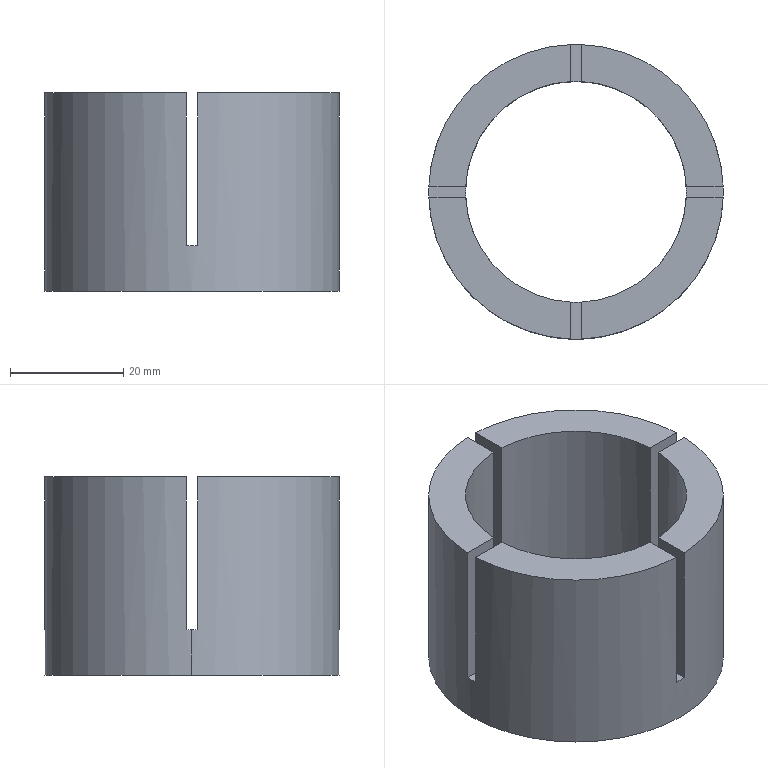Part | SolidWorks | features BaseBody 1, Cut 1 | 1 solid | 21 faces | box 52 x 52 x 35 mm | volume 31115 mm3 | plane 17 | cylinder 4 | commonest cylinder face diameters 39 x2 52 x2
STEP:
#1=CARTESIAN_POINT('',(26.,0.,11.));
#2=VERTEX_POINT('',#1);
#3=CARTESIAN_POINT('',(-26.,0.,11.));
#4=VERTEX_POINT('',#3);
#5=CARTESIAN_POINT('',(0.,0.,11.));
#6=DIRECTION('',(0.,0.,1.));
#7=DIRECTION('',(1.,0.,0.));
#8=AXIS2_PLACEMENT_3D('',#5,#6,#7);
#9=CIRCLE('',#8,26.);
#10=EDGE_CURVE('',#2,#4,#9,.T.);
#11=ORIENTED_EDGE('',*,*,#10,.T.);
#12=CARTESIAN_POINT('',(-26.,0.,19.));
#13=VERTEX_POINT('',#12);
#14=CARTESIAN_POINT('',(-26.,0.,11.));
#15=DIRECTION('',(0.,0.,1.));
#16=VECTOR('',#15,1000.);
#17=LINE('',#14,#16);
#18=EDGE_CURVE('',#4,#13,#17,.T.);
#19=ORIENTED_EDGE('',*,*,#18,.T.);
#20=CARTESIAN_POINT('',(-25.981,1.,19.));
#21=VERTEX_POINT('',#20);
#22=CARTESIAN_POINT('',(0.,0.,19.));
#23=DIRECTION('',(0.,0.,-1.));
#24=DIRECTION('',(1.,0.,0.));
#25=AXIS2_PLACEMENT_3D('',#22,#23,#24);
#26=CIRCLE('',#25,26.);
#27=EDGE_CURVE('',#13,#21,#26,.T.);
#28=ORIENTED_EDGE('',*,*,#27,.T.);
#29=CARTESIAN_POINT('',(-25.981,1.,46.));
#30=VERTEX_POINT('',#29);
#31=CARTESIAN_POINT('',(-25.981,1.,11.));
#32=DIRECTION('',(0.,0.,1.));
#33=VECTOR('',#32,1000.);
#34=LINE('',#31,#33);
#35=EDGE_CURVE('',#21,#30,#34,.T.);
#36=ORIENTED_EDGE('',*,*,#35,.T.);
#37=CARTESIAN_POINT('',(-1.,25.981,46.));
#38=VERTEX_POINT('',#37);
#39=CARTESIAN_POINT('',(0.,0.,46.));
#40=DIRECTION('',(0.,0.,-1.));
#41=DIRECTION('',(1.,0.,0.));
#42=AXIS2_PLACEMENT_3D('',#39,#40,#41);
#43=CIRCLE('',#42,26.);
#44=EDGE_CURVE('',#30,#38,#43,.T.);
#45=ORIENTED_EDGE('',*,*,#44,.T.);
#46=CARTESIAN_POINT('',(-1.,25.981,19.));
#47=VERTEX_POINT('',#46);
#48=CARTESIAN_POINT('',(-1.,25.981,11.));
#49=DIRECTION('',(0.,0.,-1.));
#50=VECTOR('',#49,1000.);
#51=LINE('',#48,#50);
#52=EDGE_CURVE('',#38,#47,#51,.T.);
#53=ORIENTED_EDGE('',*,*,#52,.T.);
#54=CARTESIAN_POINT('',(1.,25.981,19.));
#55=VERTEX_POINT('',#54);
#56=CARTESIAN_POINT('',(0.,0.,19.));
#57=DIRECTION('',(0.,0.,-1.));
#58=DIRECTION('',(1.,0.,0.));
#59=AXIS2_PLACEMENT_3D('',#56,#57,#58);
#60=CIRCLE('',#59,26.);
#61=EDGE_CURVE('',#47,#55,#60,.T.);
#62=ORIENTED_EDGE('',*,*,#61,.T.);
#63=CARTESIAN_POINT('',(1.,25.981,46.));
#64=VERTEX_POINT('',#63);
#65=CARTESIAN_POINT('',(1.,25.981,11.));
#66=DIRECTION('',(0.,0.,1.));
#67=VECTOR('',#66,1000.);
#68=LINE('',#65,#67);
#69=EDGE_CURVE('',#55,#64,#68,.T.);
#70=ORIENTED_EDGE('',*,*,#69,.T.);
#71=CARTESIAN_POINT('',(25.981,1.,46.));
#72=VERTEX_POINT('',#71);
#73=CARTESIAN_POINT('',(0.,0.,46.));
#74=DIRECTION('',(0.,0.,-1.));
#75=DIRECTION('',(1.,0.,0.));
#76=AXIS2_PLACEMENT_3D('',#73,#74,#75);
#77=CIRCLE('',#76,26.);
#78=EDGE_CURVE('',#64,#72,#77,.T.);
#79=ORIENTED_EDGE('',*,*,#78,.T.);
#80=CARTESIAN_POINT('',(25.981,1.,19.));
#81=VERTEX_POINT('',#80);
#82=CARTESIAN_POINT('',(25.981,1.,11.));
#83=DIRECTION('',(0.,0.,-1.));
#84=VECTOR('',#83,1000.);
#85=LINE('',#82,#84);
#86=EDGE_CURVE('',#72,#81,#85,.T.);
#87=ORIENTED_EDGE('',*,*,#86,.T.);
#88=CARTESIAN_POINT('',(26.,0.,19.));
#89=VERTEX_POINT('',#88);
#90=CARTESIAN_POINT('',(0.,0.,19.));
#91=DIRECTION('',(0.,0.,1.));
#92=DIRECTION('',(1.,0.,0.));
#93=AXIS2_PLACEMENT_3D('',#90,#91,#92);
#94=CIRCLE('',#93,26.);
#95=EDGE_CURVE('',#89,#81,#94,.T.);
#96=ORIENTED_EDGE('',*,*,#95,.F.);
#97=CARTESIAN_POINT('',(26.,0.,11.));
#98=DIRECTION('',(0.,0.,1.));
#99=VECTOR('',#98,1000.);
#100=LINE('',#97,#99);
#101=EDGE_CURVE('',#2,#89,#100,.T.);
#102=ORIENTED_EDGE('',*,*,#101,.F.);
#103=EDGE_LOOP('',(#11,#19,#28,#36,#45,#53,#62,#70,#79,#87,#96,#102));
#104=FACE_OUTER_BOUND('',#103,.T.);
#105=CARTESIAN_POINT('',(0.,0.,11.));
#106=DIRECTION('',(0.,0.,1.));
#107=DIRECTION('',(1.,0.,0.));
#108=AXIS2_PLACEMENT_3D('',#105,#106,#107);
#109=CYLINDRICAL_SURFACE('',#108,26.);
#110=ADVANCED_FACE('',(#104),#109,.T.);
#111=CARTESIAN_POINT('',(19.5,0.,11.));
#112=VERTEX_POINT('',#111);
#113=CARTESIAN_POINT('',(-19.5,0.,11.));
#114=VERTEX_POINT('',#113);
#115=CARTESIAN_POINT('',(0.,0.,11.));
#116=DIRECTION('',(0.,0.,-1.));
#117=DIRECTION('',(1.,0.,0.));
#118=AXIS2_PLACEMENT_3D('',#115,#116,#117);
#119=CIRCLE('',#118,19.5);
#120=EDGE_CURVE('',#112,#114,#119,.T.);
#121=ORIENTED_EDGE('',*,*,#120,.T.);
#122=CARTESIAN_POINT('',(-19.5,0.,19.));
#123=VERTEX_POINT('',#122);
#124=CARTESIAN_POINT('',(-19.5,0.,11.));
#125=DIRECTION('',(0.,0.,1.));
#126=VECTOR('',#125,1000.);
#127=LINE('',#124,#126);
#128=EDGE_CURVE('',#114,#123,#127,.T.);
#129=ORIENTED_EDGE('',*,*,#128,.T.);
#130=CARTESIAN_POINT('',(-19.474,-1.,19.));
#131=VERTEX_POINT('',#130);
#132=CARTESIAN_POINT('',(0.,0.,19.));
#133=DIRECTION('',(0.,0.,-1.));
#134=DIRECTION('',(1.,0.,0.));
#135=AXIS2_PLACEMENT_3D('',#132,#133,#134);
#136=CIRCLE('',#135,19.5);
#137=EDGE_CURVE('',#131,#123,#136,.T.);
#138=ORIENTED_EDGE('',*,*,#137,.F.);
#139=CARTESIAN_POINT('',(-19.474,-1.,46.));
#140=VERTEX_POINT('',#139);
#141=CARTESIAN_POINT('',(-19.474,-1.,19.));
#142=DIRECTION('',(0.,0.,-1.));
#143=VECTOR('',#142,1000.);
#144=LINE('',#141,#143);
#145=EDGE_CURVE('',#140,#131,#144,.T.);
#146=ORIENTED_EDGE('',*,*,#145,.F.);
#147=CARTESIAN_POINT('',(-1.,-19.474,46.));
#148=VERTEX_POINT('',#147);
#149=CARTESIAN_POINT('',(0.,0.,46.));
#150=DIRECTION('',(0.,0.,-1.));
#151=DIRECTION('',(1.,0.,0.));
#152=AXIS2_PLACEMENT_3D('',#149,#150,#151);
#153=CIRCLE('',#152,19.5);
#154=EDGE_CURVE('',#148,#140,#153,.T.);
#155=ORIENTED_EDGE('',*,*,#154,.F.);
#156=CARTESIAN_POINT('',(-1.,-19.474,19.));
#157=VERTEX_POINT('',#156);
#158=CARTESIAN_POINT('',(-1.,-19.474,19.));
#159=DIRECTION('',(0.,0.,-1.));
#160=VECTOR('',#159,1000.);
#161=LINE('',#158,#160);
#162=EDGE_CURVE('',#148,#157,#161,.T.);
#163=ORIENTED_EDGE('',*,*,#162,.T.);
#164=CARTESIAN_POINT('',(1.,-19.474,19.));
#165=VERTEX_POINT('',#164);
#166=CARTESIAN_POINT('',(0.,0.,19.));
#167=DIRECTION('',(0.,0.,-1.));
#168=DIRECTION('',(1.,0.,0.));
#169=AXIS2_PLACEMENT_3D('',#166,#167,#168);
#170=CIRCLE('',#169,19.5);
#171=EDGE_CURVE('',#165,#157,#170,.T.);
#172=ORIENTED_EDGE('',*,*,#171,.F.);
#173=CARTESIAN_POINT('',(1.,-19.474,46.));
#174=VERTEX_POINT('',#173);
#175=CARTESIAN_POINT('',(1.,-19.474,19.));
#176=DIRECTION('',(0.,0.,-1.));
#177=VECTOR('',#176,1000.);
#178=LINE('',#175,#177);
#179=EDGE_CURVE('',#174,#165,#178,.T.);
#180=ORIENTED_EDGE('',*,*,#179,.F.);
#181=CARTESIAN_POINT('',(19.474,-1.,46.));
#182=VERTEX_POINT('',#181);
#183=CARTESIAN_POINT('',(0.,0.,46.));
#184=DIRECTION('',(0.,0.,-1.));
#185=DIRECTION('',(1.,0.,0.));
#186=AXIS2_PLACEMENT_3D('',#183,#184,#185);
#187=CIRCLE('',#186,19.5);
#188=EDGE_CURVE('',#182,#174,#187,.T.);
#189=ORIENTED_EDGE('',*,*,#188,.F.);
#190=CARTESIAN_POINT('',(19.474,-1.,19.));
#191=VERTEX_POINT('',#190);
#192=CARTESIAN_POINT('',(19.474,-1.,19.));
#193=DIRECTION('',(0.,0.,1.));
#194=VECTOR('',#193,1000.);
#195=LINE('',#192,#194);
#196=EDGE_CURVE('',#191,#182,#195,.T.);
#197=ORIENTED_EDGE('',*,*,#196,.F.);
#198=CARTESIAN_POINT('',(19.5,0.,19.));
#199=VERTEX_POINT('',#198);
#200=CARTESIAN_POINT('',(0.,0.,19.));
#201=DIRECTION('',(0.,0.,-1.));
#202=DIRECTION('',(1.,0.,0.));
#203=AXIS2_PLACEMENT_3D('',#200,#201,#202);
#204=CIRCLE('',#203,19.5);
#205=EDGE_CURVE('',#199,#191,#204,.T.);
#206=ORIENTED_EDGE('',*,*,#205,.F.);
#207=CARTESIAN_POINT('',(19.5,0.,11.));
#208=DIRECTION('',(0.,0.,1.));
#209=VECTOR('',#208,1000.);
#210=LINE('',#207,#209);
#211=EDGE_CURVE('',#112,#199,#210,.T.);
#212=ORIENTED_EDGE('',*,*,#211,.F.);
#213=EDGE_LOOP('',(#121,#129,#138,#146,#155,#163,#172,#180,#189,#197,#206,#212));
#214=FACE_OUTER_BOUND('',#213,.T.);
#215=CARTESIAN_POINT('',(0.,0.,11.));
#216=DIRECTION('',(0.,0.,1.));
#217=DIRECTION('',(1.,0.,0.));
#218=AXIS2_PLACEMENT_3D('',#215,#216,#217);
#219=CYLINDRICAL_SURFACE('',#218,19.5);
#220=ADVANCED_FACE('',(#214),#219,.F.);
#221=ORIENTED_EDGE('',*,*,#18,.F.);
#222=CARTESIAN_POINT('',(0.,0.,11.));
#223=DIRECTION('',(0.,0.,1.));
#224=DIRECTION('',(1.,0.,0.));
#225=AXIS2_PLACEMENT_3D('',#222,#223,#224);
#226=CIRCLE('',#225,26.);
#227=EDGE_CURVE('',#4,#2,#226,.T.);
#228=ORIENTED_EDGE('',*,*,#227,.T.);
#229=ORIENTED_EDGE('',*,*,#101,.T.);
#230=CARTESIAN_POINT('',(25.981,-1.,19.));
#231=VERTEX_POINT('',#230);
#232=CARTESIAN_POINT('',(0.,0.,19.));
#233=DIRECTION('',(0.,0.,1.));
#234=DIRECTION('',(1.,0.,0.));
#235=AXIS2_PLACEMENT_3D('',#232,#233,#234);
#236=CIRCLE('',#235,26.);
#237=EDGE_CURVE('',#231,#89,#236,.T.);
#238=ORIENTED_EDGE('',*,*,#237,.F.);
#239=CARTESIAN_POINT('',(25.981,-1.,46.));
#240=VERTEX_POINT('',#239);
#241=CARTESIAN_POINT('',(25.981,-1.,11.));
#242=DIRECTION('',(0.,0.,1.));
#243=VECTOR('',#242,1000.);
#244=LINE('',#241,#243);
#245=EDGE_CURVE('',#231,#240,#244,.T.);
#246=ORIENTED_EDGE('',*,*,#245,.T.);
#247=CARTESIAN_POINT('',(1.,-25.981,46.));
#248=VERTEX_POINT('',#247);
#249=CARTESIAN_POINT('',(0.,0.,46.));
#250=DIRECTION('',(0.,0.,-1.));
#251=DIRECTION('',(1.,0.,0.));
#252=AXIS2_PLACEMENT_3D('',#249,#250,#251);
#253=CIRCLE('',#252,26.);
#254=EDGE_CURVE('',#240,#248,#253,.T.);
#255=ORIENTED_EDGE('',*,*,#254,.T.);
#256=CARTESIAN_POINT('',(1.,-25.981,19.));
#257=VERTEX_POINT('',#256);
#258=CARTESIAN_POINT('',(1.,-25.981,11.));
#259=DIRECTION('',(0.,0.,-1.));
#260=VECTOR('',#259,1000.);
#261=LINE('',#258,#260);
#262=EDGE_CURVE('',#248,#257,#261,.T.);
#263=ORIENTED_EDGE('',*,*,#262,.T.);
#264=CARTESIAN_POINT('',(-1.,-25.981,19.));
#265=VERTEX_POINT('',#264);
#266=CARTESIAN_POINT('',(0.,0.,19.));
#267=DIRECTION('',(0.,0.,-1.));
#268=DIRECTION('',(1.,0.,0.));
#269=AXIS2_PLACEMENT_3D('',#266,#267,#268);
#270=CIRCLE('',#269,26.);
#271=EDGE_CURVE('',#257,#265,#270,.T.);
#272=ORIENTED_EDGE('',*,*,#271,.T.);
#273=CARTESIAN_POINT('',(-1.,-25.981,46.));
#274=VERTEX_POINT('',#273);
#275=CARTESIAN_POINT('',(-1.,-25.981,11.));
#276=DIRECTION('',(0.,0.,1.));
#277=VECTOR('',#276,1000.);
#278=LINE('',#275,#277);
#279=EDGE_CURVE('',#265,#274,#278,.T.);
#280=ORIENTED_EDGE('',*,*,#279,.T.);
#281=CARTESIAN_POINT('',(-25.981,-1.,46.));
#282=VERTEX_POINT('',#281);
#283=CARTESIAN_POINT('',(0.,0.,46.));
#284=DIRECTION('',(0.,0.,-1.));
#285=DIRECTION('',(1.,0.,0.));
#286=AXIS2_PLACEMENT_3D('',#283,#284,#285);
#287=CIRCLE('',#286,26.);
#288=EDGE_CURVE('',#274,#282,#287,.T.);
#289=ORIENTED_EDGE('',*,*,#288,.T.);
#290=CARTESIAN_POINT('',(-25.981,-1.,19.));
#291=VERTEX_POINT('',#290);
#292=CARTESIAN_POINT('',(-25.981,-1.,11.));
#293=DIRECTION('',(0.,0.,-1.));
#294=VECTOR('',#293,1000.);
#295=LINE('',#292,#294);
#296=EDGE_CURVE('',#282,#291,#295,.T.);
#297=ORIENTED_EDGE('',*,*,#296,.T.);
#298=CARTESIAN_POINT('',(0.,0.,19.));
#299=DIRECTION('',(0.,0.,-1.));
#300=DIRECTION('',(1.,0.,0.));
#301=AXIS2_PLACEMENT_3D('',#298,#299,#300);
#302=CIRCLE('',#301,26.);
#303=EDGE_CURVE('',#291,#13,#302,.T.);
#304=ORIENTED_EDGE('',*,*,#303,.T.);
#305=EDGE_LOOP('',(#221,#228,#229,#238,#246,#255,#263,#272,#280,#289,#297,#304));
#306=FACE_OUTER_BOUND('',#305,.T.);
#307=CARTESIAN_POINT('',(0.,0.,11.));
#308=DIRECTION('',(0.,0.,1.));
#309=DIRECTION('',(1.,0.,0.));
#310=AXIS2_PLACEMENT_3D('',#307,#308,#309);
#311=CYLINDRICAL_SURFACE('',#310,26.);
#312=ADVANCED_FACE('',(#306),#311,.T.);
#313=CARTESIAN_POINT('',(19.474,1.,46.));
#314=VERTEX_POINT('',#313);
#315=CARTESIAN_POINT('',(-36.,1.,46.));
#316=DIRECTION('',(1.,0.,0.));
#317=VECTOR('',#316,1000.);
#318=LINE('',#315,#317);
#319=EDGE_CURVE('',#314,#72,#318,.T.);
#320=ORIENTED_EDGE('',*,*,#319,.F.);
#321=CARTESIAN_POINT('',(19.474,1.,19.));
#322=VERTEX_POINT('',#321);
#323=CARTESIAN_POINT('',(19.474,1.,19.));
#324=DIRECTION('',(0.,0.,1.));
#325=VECTOR('',#324,1000.);
#326=LINE('',#323,#325);
#327=EDGE_CURVE('',#322,#314,#326,.T.);
#328=ORIENTED_EDGE('',*,*,#327,.F.);
#329=CARTESIAN_POINT('',(-36.,1.,19.));
#330=DIRECTION('',(-1.,0.,0.));
#331=VECTOR('',#330,1000.);
#332=LINE('',#329,#331);
#333=EDGE_CURVE('',#81,#322,#332,.T.);
#334=ORIENTED_EDGE('',*,*,#333,.F.);
#335=ORIENTED_EDGE('',*,*,#86,.F.);
#336=EDGE_LOOP('',(#320,#328,#334,#335));
#337=FACE_OUTER_BOUND('',#336,.T.);
#338=CARTESIAN_POINT('',(-36.,1.,19.));
#339=DIRECTION('',(0.,1.,0.));
#340=DIRECTION('',(0.,0.,1.));
#341=AXIS2_PLACEMENT_3D('',#338,#339,#340);
#342=PLANE('',#341);
#343=ADVANCED_FACE('',(#337),#342,.F.);
#344=CARTESIAN_POINT('',(1.,19.474,46.));
#345=VERTEX_POINT('',#344);
#346=CARTESIAN_POINT('',(1.,0.,46.));
#347=DIRECTION('',(0.,-1.,0.));
#348=VECTOR('',#347,1000.);
#349=LINE('',#346,#348);
#350=EDGE_CURVE('',#64,#345,#349,.T.);
#351=ORIENTED_EDGE('',*,*,#350,.T.);
#352=CARTESIAN_POINT('',(0.,0.,46.));
#353=DIRECTION('',(0.,0.,-1.));
#354=DIRECTION('',(1.,0.,0.));
#355=AXIS2_PLACEMENT_3D('',#352,#353,#354);
#356=CIRCLE('',#355,19.5);
#357=EDGE_CURVE('',#345,#314,#356,.T.);
#358=ORIENTED_EDGE('',*,*,#357,.T.);
#359=ORIENTED_EDGE('',*,*,#319,.T.);
#360=ORIENTED_EDGE('',*,*,#78,.F.);
#361=EDGE_LOOP('',(#351,#358,#359,#360));
#362=FACE_OUTER_BOUND('',#361,.T.);
#363=CARTESIAN_POINT('',(0.,0.,46.));
#364=DIRECTION('',(0.,0.,1.));
#365=DIRECTION('',(1.,0.,0.));
#366=AXIS2_PLACEMENT_3D('',#363,#364,#365);
#367=PLANE('',#366);
#368=ADVANCED_FACE('',(#362),#367,.T.);
#369=ORIENTED_EDGE('',*,*,#350,.F.);
#370=ORIENTED_EDGE('',*,*,#69,.F.);
#371=CARTESIAN_POINT('',(1.,19.474,19.));
#372=VERTEX_POINT('',#371);
#373=CARTESIAN_POINT('',(1.,-42.,19.));
#374=DIRECTION('',(0.,-1.,0.));
#375=VECTOR('',#374,1000.);
#376=LINE('',#373,#375);
#377=EDGE_CURVE('',#55,#372,#376,.T.);
#378=ORIENTED_EDGE('',*,*,#377,.T.);
#379=CARTESIAN_POINT('',(1.,19.474,19.));
#380=DIRECTION('',(0.,0.,1.));
#381=VECTOR('',#380,1000.);
#382=LINE('',#379,#381);
#383=EDGE_CURVE('',#372,#345,#382,.T.);
#384=ORIENTED_EDGE('',*,*,#383,.T.);
#385=EDGE_LOOP('',(#369,#370,#378,#384));
#386=FACE_OUTER_BOUND('',#385,.T.);
#387=CARTESIAN_POINT('',(1.,-42.,19.));
#388=DIRECTION('',(-1.,0.,0.));
#389=DIRECTION('',(0.,-1.,0.));
#390=AXIS2_PLACEMENT_3D('',#387,#388,#389);
#391=PLANE('',#390);
#392=ADVANCED_FACE('',(#386),#391,.T.);
#393=ORIENTED_EDGE('',*,*,#377,.F.);
#394=ORIENTED_EDGE('',*,*,#61,.F.);
#395=CARTESIAN_POINT('',(-1.,19.474,19.));
#396=VERTEX_POINT('',#395);
#397=CARTESIAN_POINT('',(-1.,-42.,19.));
#398=DIRECTION('',(0.,-1.,0.));
#399=VECTOR('',#398,1000.);
#400=LINE('',#397,#399);
#401=EDGE_CURVE('',#47,#396,#400,.T.);
#402=ORIENTED_EDGE('',*,*,#401,.T.);
#403=CARTESIAN_POINT('',(0.,0.,19.));
#404=DIRECTION('',(0.,0.,-1.));
#405=DIRECTION('',(1.,0.,0.));
#406=AXIS2_PLACEMENT_3D('',#403,#404,#405);
#407=CIRCLE('',#406,19.5);
#408=EDGE_CURVE('',#396,#372,#407,.T.);
#409=ORIENTED_EDGE('',*,*,#408,.T.);
#410=EDGE_LOOP('',(#393,#394,#402,#409));
#411=FACE_OUTER_BOUND('',#410,.T.);
#412=CARTESIAN_POINT('',(1.,-42.,19.));
#413=DIRECTION('',(0.,0.,1.));
#414=DIRECTION('',(1.,0.,0.));
#415=AXIS2_PLACEMENT_3D('',#412,#413,#414);
#416=PLANE('',#415);
#417=ADVANCED_FACE('',(#411),#416,.T.);
#418=CARTESIAN_POINT('',(-1.,19.474,46.));
#419=VERTEX_POINT('',#418);
#420=CARTESIAN_POINT('',(-1.,-42.,46.));
#421=DIRECTION('',(0.,1.,0.));
#422=VECTOR('',#421,1000.);
#423=LINE('',#420,#422);
#424=EDGE_CURVE('',#419,#38,#423,.T.);
#425=ORIENTED_EDGE('',*,*,#424,.F.);
#426=CARTESIAN_POINT('',(-1.,19.474,19.));
#427=DIRECTION('',(0.,0.,1.));
#428=VECTOR('',#427,1000.);
#429=LINE('',#426,#428);
#430=EDGE_CURVE('',#396,#419,#429,.T.);
#431=ORIENTED_EDGE('',*,*,#430,.F.);
#432=ORIENTED_EDGE('',*,*,#401,.F.);
#433=ORIENTED_EDGE('',*,*,#52,.F.);
#434=EDGE_LOOP('',(#425,#431,#432,#433));
#435=FACE_OUTER_BOUND('',#434,.T.);
#436=CARTESIAN_POINT('',(-1.,-42.,19.));
#437=DIRECTION('',(-1.,0.,0.));
#438=DIRECTION('',(0.,-1.,0.));
#439=AXIS2_PLACEMENT_3D('',#436,#437,#438);
#440=PLANE('',#439);
#441=ADVANCED_FACE('',(#435),#440,.F.);
#442=CARTESIAN_POINT('',(-19.474,1.,46.));
#443=VERTEX_POINT('',#442);
#444=CARTESIAN_POINT('',(0.,1.,46.));
#445=DIRECTION('',(1.,0.,0.));
#446=VECTOR('',#445,1000.);
#447=LINE('',#444,#446);
#448=EDGE_CURVE('',#30,#443,#447,.T.);
#449=ORIENTED_EDGE('',*,*,#448,.T.);
#450=CARTESIAN_POINT('',(0.,0.,46.));
#451=DIRECTION('',(0.,0.,-1.));
#452=DIRECTION('',(1.,0.,0.));
#453=AXIS2_PLACEMENT_3D('',#450,#451,#452);
#454=CIRCLE('',#453,19.5);
#455=EDGE_CURVE('',#443,#419,#454,.T.);
#456=ORIENTED_EDGE('',*,*,#455,.T.);
#457=ORIENTED_EDGE('',*,*,#424,.T.);
#458=ORIENTED_EDGE('',*,*,#44,.F.);
#459=EDGE_LOOP('',(#449,#456,#457,#458));
#460=FACE_OUTER_BOUND('',#459,.T.);
#461=CARTESIAN_POINT('',(0.,0.,46.));
#462=DIRECTION('',(0.,0.,1.));
#463=DIRECTION('',(1.,0.,0.));
#464=AXIS2_PLACEMENT_3D('',#461,#462,#463);
#465=PLANE('',#464);
#466=ADVANCED_FACE('',(#460),#465,.T.);
#467=ORIENTED_EDGE('',*,*,#448,.F.);
#468=ORIENTED_EDGE('',*,*,#35,.F.);
#469=CARTESIAN_POINT('',(-19.474,1.,19.));
#470=VERTEX_POINT('',#469);
#471=CARTESIAN_POINT('',(-36.,1.,19.));
#472=DIRECTION('',(-1.,0.,0.));
#473=VECTOR('',#472,1000.);
#474=LINE('',#471,#473);
#475=EDGE_CURVE('',#470,#21,#474,.T.);
#476=ORIENTED_EDGE('',*,*,#475,.F.);
#477=CARTESIAN_POINT('',(-19.474,1.,19.));
#478=DIRECTION('',(0.,0.,-1.));
#479=VECTOR('',#478,1000.);
#480=LINE('',#477,#479);
#481=EDGE_CURVE('',#443,#470,#480,.T.);
#482=ORIENTED_EDGE('',*,*,#481,.F.);
#483=EDGE_LOOP('',(#467,#468,#476,#482));
#484=FACE_OUTER_BOUND('',#483,.T.);
#485=CARTESIAN_POINT('',(-36.,1.,19.));
#486=DIRECTION('',(0.,1.,0.));
#487=DIRECTION('',(0.,0.,1.));
#488=AXIS2_PLACEMENT_3D('',#485,#486,#487);
#489=PLANE('',#488);
#490=ADVANCED_FACE('',(#484),#489,.F.);
#491=CARTESIAN_POINT('',(-36.,-1.,19.));
#492=DIRECTION('',(1.,0.,0.));
#493=VECTOR('',#492,1000.);
#494=LINE('',#491,#493);
#495=EDGE_CURVE('',#291,#131,#494,.T.);
#496=ORIENTED_EDGE('',*,*,#495,.T.);
#497=ORIENTED_EDGE('',*,*,#137,.T.);
#498=CARTESIAN_POINT('',(0.,0.,19.));
#499=DIRECTION('',(0.,0.,-1.));
#500=DIRECTION('',(1.,0.,0.));
#501=AXIS2_PLACEMENT_3D('',#498,#499,#500);
#502=CIRCLE('',#501,19.5);
#503=EDGE_CURVE('',#123,#470,#502,.T.);
#504=ORIENTED_EDGE('',*,*,#503,.T.);
#505=ORIENTED_EDGE('',*,*,#475,.T.);
#506=ORIENTED_EDGE('',*,*,#27,.F.);
#507=ORIENTED_EDGE('',*,*,#303,.F.);
#508=EDGE_LOOP('',(#496,#497,#504,#505,#506,#507));
#509=FACE_OUTER_BOUND('',#508,.T.);
#510=CARTESIAN_POINT('',(-36.,-1.,19.));
#511=DIRECTION('',(0.,0.,1.));
#512=DIRECTION('',(1.,0.,0.));
#513=AXIS2_PLACEMENT_3D('',#510,#511,#512);
#514=PLANE('',#513);
#515=ADVANCED_FACE('',(#509),#514,.T.);
#516=CARTESIAN_POINT('',(-36.,-1.,46.));
#517=DIRECTION('',(1.,0.,0.));
#518=VECTOR('',#517,1000.);
#519=LINE('',#516,#518);
#520=EDGE_CURVE('',#282,#140,#519,.T.);
#521=ORIENTED_EDGE('',*,*,#520,.T.);
#522=ORIENTED_EDGE('',*,*,#145,.T.);
#523=ORIENTED_EDGE('',*,*,#495,.F.);
#524=ORIENTED_EDGE('',*,*,#296,.F.);
#525=EDGE_LOOP('',(#521,#522,#523,#524));
#526=FACE_OUTER_BOUND('',#525,.T.);
#527=CARTESIAN_POINT('',(-36.,-1.,19.));
#528=DIRECTION('',(0.,1.,0.));
#529=DIRECTION('',(0.,0.,1.));
#530=AXIS2_PLACEMENT_3D('',#527,#528,#529);
#531=PLANE('',#530);
#532=ADVANCED_FACE('',(#526),#531,.T.);
#533=CARTESIAN_POINT('',(-1.,0.,46.));
#534=DIRECTION('',(0.,1.,0.));
#535=VECTOR('',#534,1000.);
#536=LINE('',#533,#535);
#537=EDGE_CURVE('',#274,#148,#536,.T.);
#538=ORIENTED_EDGE('',*,*,#537,.T.);
#539=ORIENTED_EDGE('',*,*,#154,.T.);
#540=ORIENTED_EDGE('',*,*,#520,.F.);
#541=ORIENTED_EDGE('',*,*,#288,.F.);
#542=EDGE_LOOP('',(#538,#539,#540,#541));
#543=FACE_OUTER_BOUND('',#542,.T.);
#544=CARTESIAN_POINT('',(0.,0.,46.));
#545=DIRECTION('',(0.,0.,1.));
#546=DIRECTION('',(1.,0.,0.));
#547=AXIS2_PLACEMENT_3D('',#544,#545,#546);
#548=PLANE('',#547);
#549=ADVANCED_FACE('',(#543),#548,.T.);
#550=ORIENTED_EDGE('',*,*,#537,.F.);
#551=ORIENTED_EDGE('',*,*,#279,.F.);
#552=CARTESIAN_POINT('',(-1.,-42.,19.));
#553=DIRECTION('',(0.,-1.,0.));
#554=VECTOR('',#553,1000.);
#555=LINE('',#552,#554);
#556=EDGE_CURVE('',#157,#265,#555,.T.);
#557=ORIENTED_EDGE('',*,*,#556,.F.);
#558=ORIENTED_EDGE('',*,*,#162,.F.);
#559=EDGE_LOOP('',(#550,#551,#557,#558));
#560=FACE_OUTER_BOUND('',#559,.T.);
#561=CARTESIAN_POINT('',(-1.,-42.,19.));
#562=DIRECTION('',(-1.,0.,0.));
#563=DIRECTION('',(0.,-1.,0.));
#564=AXIS2_PLACEMENT_3D('',#561,#562,#563);
#565=PLANE('',#564);
#566=ADVANCED_FACE('',(#560),#565,.F.);
#567=CARTESIAN_POINT('',(1.,-42.,19.));
#568=DIRECTION('',(0.,1.,0.));
#569=VECTOR('',#568,1000.);
#570=LINE('',#567,#569);
#571=EDGE_CURVE('',#257,#165,#570,.T.);
#572=ORIENTED_EDGE('',*,*,#571,.T.);
#573=ORIENTED_EDGE('',*,*,#171,.T.);
#574=ORIENTED_EDGE('',*,*,#556,.T.);
#575=ORIENTED_EDGE('',*,*,#271,.F.);
#576=EDGE_LOOP('',(#572,#573,#574,#575));
#577=FACE_OUTER_BOUND('',#576,.T.);
#578=CARTESIAN_POINT('',(1.,-42.,19.));
#579=DIRECTION('',(0.,0.,1.));
#580=DIRECTION('',(1.,0.,0.));
#581=AXIS2_PLACEMENT_3D('',#578,#579,#580);
#582=PLANE('',#581);
#583=ADVANCED_FACE('',(#577),#582,.T.);
#584=CARTESIAN_POINT('',(1.,-42.,46.));
#585=DIRECTION('',(0.,1.,0.));
#586=VECTOR('',#585,1000.);
#587=LINE('',#584,#586);
#588=EDGE_CURVE('',#248,#174,#587,.T.);
#589=ORIENTED_EDGE('',*,*,#588,.T.);
#590=ORIENTED_EDGE('',*,*,#179,.T.);
#591=ORIENTED_EDGE('',*,*,#571,.F.);
#592=ORIENTED_EDGE('',*,*,#262,.F.);
#593=EDGE_LOOP('',(#589,#590,#591,#592));
#594=FACE_OUTER_BOUND('',#593,.T.);
#595=CARTESIAN_POINT('',(1.,-42.,19.));
#596=DIRECTION('',(-1.,0.,0.));
#597=DIRECTION('',(0.,-1.,0.));
#598=AXIS2_PLACEMENT_3D('',#595,#596,#597);
#599=PLANE('',#598);
#600=ADVANCED_FACE('',(#594),#599,.T.);
#601=CARTESIAN_POINT('',(0.,-1.,46.));
#602=DIRECTION('',(-1.,0.,0.));
#603=VECTOR('',#602,1000.);
#604=LINE('',#601,#603);
#605=EDGE_CURVE('',#240,#182,#604,.T.);
#606=ORIENTED_EDGE('',*,*,#605,.T.);
#607=ORIENTED_EDGE('',*,*,#188,.T.);
#608=ORIENTED_EDGE('',*,*,#588,.F.);
#609=ORIENTED_EDGE('',*,*,#254,.F.);
#610=EDGE_LOOP('',(#606,#607,#608,#609));
#611=FACE_OUTER_BOUND('',#610,.T.);
#612=CARTESIAN_POINT('',(0.,0.,46.));
#613=DIRECTION('',(0.,0.,1.));
#614=DIRECTION('',(1.,0.,0.));
#615=AXIS2_PLACEMENT_3D('',#612,#613,#614);
#616=PLANE('',#615);
#617=ADVANCED_FACE('',(#611),#616,.T.);
#618=ORIENTED_EDGE('',*,*,#605,.F.);
#619=ORIENTED_EDGE('',*,*,#245,.F.);
#620=CARTESIAN_POINT('',(-36.,-1.,19.));
#621=DIRECTION('',(-1.,0.,0.));
#622=VECTOR('',#621,1000.);
#623=LINE('',#620,#622);
#624=EDGE_CURVE('',#231,#191,#623,.T.);
#625=ORIENTED_EDGE('',*,*,#624,.T.);
#626=ORIENTED_EDGE('',*,*,#196,.T.);
#627=EDGE_LOOP('',(#618,#619,#625,#626));
#628=FACE_OUTER_BOUND('',#627,.T.);
#629=CARTESIAN_POINT('',(-36.,-1.,19.));
#630=DIRECTION('',(0.,1.,0.));
#631=DIRECTION('',(0.,0.,1.));
#632=AXIS2_PLACEMENT_3D('',#629,#630,#631);
#633=PLANE('',#632);
#634=ADVANCED_FACE('',(#628),#633,.T.);
#635=ORIENTED_EDGE('',*,*,#120,.F.);
#636=CARTESIAN_POINT('',(0.,0.,11.));
#637=DIRECTION('',(0.,0.,-1.));
#638=DIRECTION('',(1.,0.,0.));
#639=AXIS2_PLACEMENT_3D('',#636,#637,#638);
#640=CIRCLE('',#639,19.5);
#641=EDGE_CURVE('',#114,#112,#640,.T.);
#642=ORIENTED_EDGE('',*,*,#641,.F.);
#643=EDGE_LOOP('',(#635,#642));
#644=FACE_BOUND('',#643,.T.);
#645=ORIENTED_EDGE('',*,*,#10,.F.);
#646=ORIENTED_EDGE('',*,*,#227,.F.);
#647=EDGE_LOOP('',(#645,#646));
#648=FACE_OUTER_BOUND('',#647,.T.);
#649=CARTESIAN_POINT('',(0.,0.,11.));
#650=DIRECTION('',(0.,0.,1.));
#651=DIRECTION('',(1.,0.,0.));
#652=AXIS2_PLACEMENT_3D('',#649,#650,#651);
#653=PLANE('',#652);
#654=ADVANCED_FACE('',(#644,#648),#653,.F.);
#655=ORIENTED_EDGE('',*,*,#128,.F.);
#656=ORIENTED_EDGE('',*,*,#641,.T.);
#657=ORIENTED_EDGE('',*,*,#211,.T.);
#658=CARTESIAN_POINT('',(0.,0.,19.));
#659=DIRECTION('',(0.,0.,-1.));
#660=DIRECTION('',(1.,0.,0.));
#661=AXIS2_PLACEMENT_3D('',#658,#659,#660);
#662=CIRCLE('',#661,19.5);
#663=EDGE_CURVE('',#322,#199,#662,.T.);
#664=ORIENTED_EDGE('',*,*,#663,.F.);
#665=ORIENTED_EDGE('',*,*,#327,.T.);
#666=ORIENTED_EDGE('',*,*,#357,.F.);
#667=ORIENTED_EDGE('',*,*,#383,.F.);
#668=ORIENTED_EDGE('',*,*,#408,.F.);
#669=ORIENTED_EDGE('',*,*,#430,.T.);
#670=ORIENTED_EDGE('',*,*,#455,.F.);
#671=ORIENTED_EDGE('',*,*,#481,.T.);
#672=ORIENTED_EDGE('',*,*,#503,.F.);
#673=EDGE_LOOP('',(#655,#656,#657,#664,#665,#666,#667,#668,#669,#670,#671,#672));
#674=FACE_OUTER_BOUND('',#673,.T.);
#675=CARTESIAN_POINT('',(0.,0.,11.));
#676=DIRECTION('',(0.,0.,1.));
#677=DIRECTION('',(1.,0.,0.));
#678=AXIS2_PLACEMENT_3D('',#675,#676,#677);
#679=CYLINDRICAL_SURFACE('',#678,19.5);
#680=ADVANCED_FACE('',(#674),#679,.F.);
#681=ORIENTED_EDGE('',*,*,#624,.F.);
#682=ORIENTED_EDGE('',*,*,#237,.T.);
#683=ORIENTED_EDGE('',*,*,#95,.T.);
#684=ORIENTED_EDGE('',*,*,#333,.T.);
#685=ORIENTED_EDGE('',*,*,#663,.T.);
#686=ORIENTED_EDGE('',*,*,#205,.T.);
#687=EDGE_LOOP('',(#681,#682,#683,#684,#685,#686));
#688=FACE_OUTER_BOUND('',#687,.T.);
#689=CARTESIAN_POINT('',(-36.,-1.,19.));
#690=DIRECTION('',(0.,0.,1.));
#691=DIRECTION('',(1.,0.,0.));
#692=AXIS2_PLACEMENT_3D('',#689,#690,#691);
#693=PLANE('',#692);
#694=ADVANCED_FACE('',(#688),#693,.T.);
#695=CLOSED_SHELL('',(#110,#220,#312,#343,#368,#392,#417,#441,#466,#490,#515,#532,#549,#566,#583,#600,#617,#634,#654,#680,#694));
#696=MANIFOLD_SOLID_BREP('',#695);
#697=CARTESIAN_POINT('',(0.,0.,0.));
#698=DIRECTION('',(0.,0.,1.));
#699=DIRECTION('',(1.,0.,0.));
#700=AXIS2_PLACEMENT_3D('',#697,#698,#699);
#701=(LENGTH_UNIT()NAMED_UNIT(*)SI_UNIT(.MILLI.,.METRE.));
#702=UNCERTAINTY_MEASURE_WITH_UNIT(LENGTH_MEASURE(0.00001),#701,'','');
#703=(NAMED_UNIT(*)PLANE_ANGLE_UNIT()SI_UNIT($,.RADIAN.));
#704=(NAMED_UNIT(*)SI_UNIT($,.STERADIAN.)SOLID_ANGLE_UNIT());
#705=(GEOMETRIC_REPRESENTATION_CONTEXT(3)GLOBAL_UNCERTAINTY_ASSIGNED_CONTEXT((#702))GLOBAL_UNIT_ASSIGNED_CONTEXT((#701,#703,#704))REPRESENTATION_CONTEXT('',''));
#706=ADVANCED_BREP_SHAPE_REPRESENTATION('',(#696,#700),#705);